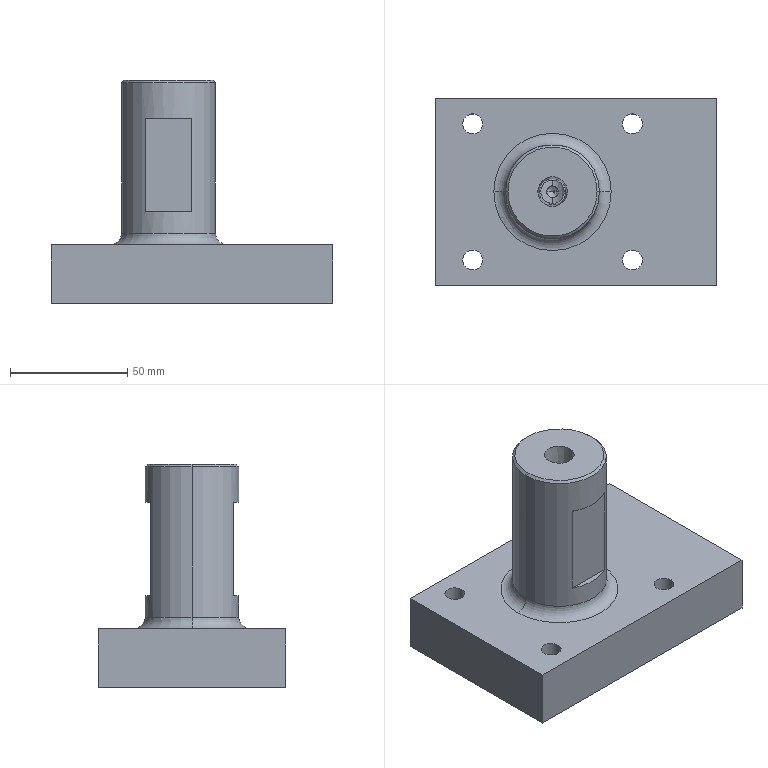Part | SolidWorks | features HoleWzd 5, ICE 4, Chamfer 1, Extrusion 1, Fillet 1, RevCut 1 | 1 solid | 54 faces | box 120 x 80 x 95 mm | volume 309106 mm3 | cylinder 24 | cone 14 | plane 14 | torus 2 | commonest cylinder face diameters 8.5 x12 5 x4 11.8 x4 10 x2 40 x2